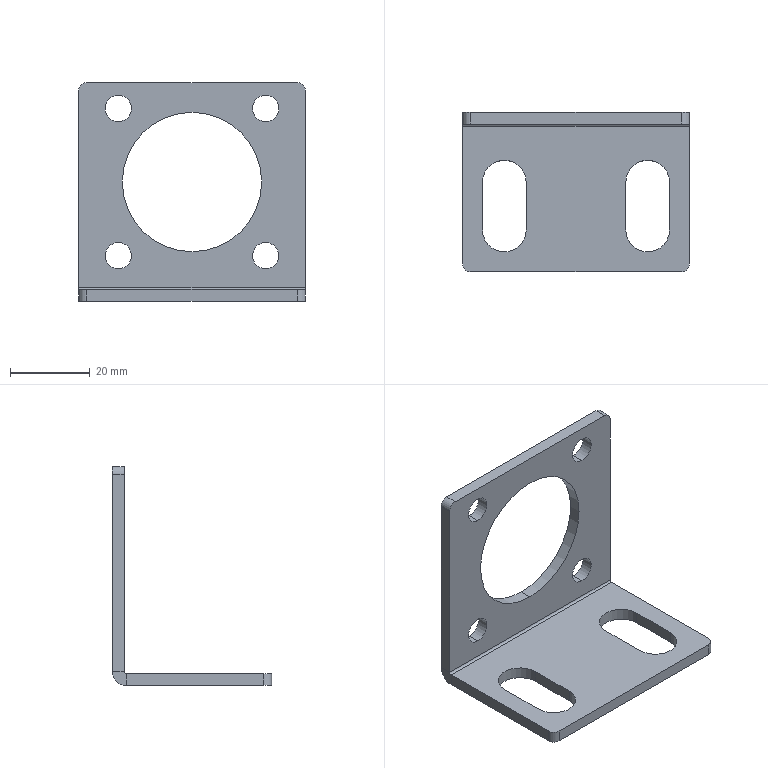Part | SolidWorks | features BaseBody 1 | 1 solid | 36 faces | box 57 x 40 x 55 mm | volume 10916 mm3 | cylinder 20 | plane 16 | commonest cylinder face diameters 6.6 x8 4 x4 11 x4 35 x2 1 x1 7 x1
STEP:
#1=CARTESIAN_POINT('',(0.,17.,9.5));
#2=VERTEX_POINT('',#1);
#3=CARTESIAN_POINT('',(0.,20.,9.5));
#4=VERTEX_POINT('',#3);
#5=CARTESIAN_POINT('',(0.,-20.,9.5));
#6=DIRECTION('',(0.,1.,0.));
#7=VECTOR('',#6,1000.);
#8=LINE('',#5,#7);
#9=EDGE_CURVE('',#2,#4,#8,.T.);
#10=ORIENTED_EDGE('',*,*,#9,.F.);
#11=CARTESIAN_POINT('',(0.,17.,44.5));
#12=VERTEX_POINT('',#11);
#13=CARTESIAN_POINT('',(0.,17.,27.));
#14=DIRECTION('',(0.,1.,0.));
#15=DIRECTION('',(0.,0.,-1.));
#16=AXIS2_PLACEMENT_3D('',#13,#14,#15);
#17=CIRCLE('',#16,17.5);
#18=EDGE_CURVE('',#12,#2,#17,.T.);
#19=ORIENTED_EDGE('',*,*,#18,.F.);
#20=CARTESIAN_POINT('',(0.,20.,44.5));
#21=VERTEX_POINT('',#20);
#22=CARTESIAN_POINT('',(0.,-20.,44.5));
#23=DIRECTION('',(0.,1.,0.));
#24=VECTOR('',#23,1000.);
#25=LINE('',#22,#24);
#26=EDGE_CURVE('',#12,#21,#25,.T.);
#27=ORIENTED_EDGE('',*,*,#26,.T.);
#28=CARTESIAN_POINT('',(0.,20.,27.));
#29=DIRECTION('',(0.,1.,0.));
#30=DIRECTION('',(0.,0.,-1.));
#31=AXIS2_PLACEMENT_3D('',#28,#29,#30);
#32=CIRCLE('',#31,17.5);
#33=EDGE_CURVE('',#21,#4,#32,.T.);
#34=ORIENTED_EDGE('',*,*,#33,.T.);
#35=EDGE_LOOP('',(#10,#19,#27,#34));
#36=FACE_OUTER_BOUND('',#35,.T.);
#37=CARTESIAN_POINT('',(0.,-20.,27.));
#38=DIRECTION('',(0.,1.,0.));
#39=DIRECTION('',(0.,0.,1.));
#40=AXIS2_PLACEMENT_3D('',#37,#38,#39);
#41=CYLINDRICAL_SURFACE('',#40,17.5);
#42=ADVANCED_FACE('',(#36),#41,.F.);
#43=CARTESIAN_POINT('',(-12.5,-9.5,0.));
#44=VERTEX_POINT('',#43);
#45=CARTESIAN_POINT('',(-12.5,-9.5,-3.));
#46=VERTEX_POINT('',#45);
#47=CARTESIAN_POINT('',(-12.5,-9.5,-3.001));
#48=DIRECTION('',(0.,0.,-1.));
#49=VECTOR('',#48,1000.);
#50=LINE('',#47,#49);
#51=EDGE_CURVE('',#44,#46,#50,.T.);
#52=ORIENTED_EDGE('',*,*,#51,.F.);
#53=CARTESIAN_POINT('',(-12.5,2.5,0.));
#54=VERTEX_POINT('',#53);
#55=CARTESIAN_POINT('',(-12.5,-9.5,0.));
#56=DIRECTION('',(0.,1.,0.));
#57=VECTOR('',#56,1000.);
#58=LINE('',#55,#57);
#59=EDGE_CURVE('',#44,#54,#58,.T.);
#60=ORIENTED_EDGE('',*,*,#59,.T.);
#61=CARTESIAN_POINT('',(-12.5,2.5,-3.));
#62=VERTEX_POINT('',#61);
#63=CARTESIAN_POINT('',(-12.5,2.5,-3.001));
#64=DIRECTION('',(0.,0.,-1.));
#65=VECTOR('',#64,1000.);
#66=LINE('',#63,#65);
#67=EDGE_CURVE('',#54,#62,#66,.T.);
#68=ORIENTED_EDGE('',*,*,#67,.T.);
#69=CARTESIAN_POINT('',(-12.5,0.,-3.));
#70=DIRECTION('',(0.,1.,0.));
#71=VECTOR('',#70,1000.);
#72=LINE('',#69,#71);
#73=EDGE_CURVE('',#46,#62,#72,.T.);
#74=ORIENTED_EDGE('',*,*,#73,.F.);
#75=EDGE_LOOP('',(#52,#60,#68,#74));
#76=FACE_OUTER_BOUND('',#75,.T.);
#77=CARTESIAN_POINT('',(-12.5,-9.5,-3.001));
#78=DIRECTION('',(1.,0.,0.));
#79=DIRECTION('',(0.,0.,1.));
#80=AXIS2_PLACEMENT_3D('',#77,#78,#79);
#81=PLANE('',#80);
#82=ADVANCED_FACE('',(#76),#81,.F.);
#83=CARTESIAN_POINT('',(-23.5,2.5,-3.));
#84=VERTEX_POINT('',#83);
#85=CARTESIAN_POINT('',(-23.5,2.5,0.));
#86=VERTEX_POINT('',#85);
#87=CARTESIAN_POINT('',(-23.5,2.5,0.));
#88=DIRECTION('',(0.,0.,1.));
#89=VECTOR('',#88,1000.);
#90=LINE('',#87,#89);
#91=EDGE_CURVE('',#84,#86,#90,.T.);
#92=ORIENTED_EDGE('',*,*,#91,.T.);
#93=CARTESIAN_POINT('',(-23.5,-9.5,0.));
#94=VERTEX_POINT('',#93);
#95=CARTESIAN_POINT('',(-23.5,-9.5,0.));
#96=DIRECTION('',(0.,1.,0.));
#97=VECTOR('',#96,1000.);
#98=LINE('',#95,#97);
#99=EDGE_CURVE('',#94,#86,#98,.T.);
#100=ORIENTED_EDGE('',*,*,#99,.F.);
#101=CARTESIAN_POINT('',(-23.5,-9.5,-3.));
#102=VERTEX_POINT('',#101);
#103=CARTESIAN_POINT('',(-23.5,-9.5,0.));
#104=DIRECTION('',(0.,0.,-1.));
#105=VECTOR('',#104,1000.);
#106=LINE('',#103,#105);
#107=EDGE_CURVE('',#94,#102,#106,.T.);
#108=ORIENTED_EDGE('',*,*,#107,.T.);
#109=CARTESIAN_POINT('',(-23.5,0.,-3.));
#110=DIRECTION('',(0.,-1.,0.));
#111=VECTOR('',#110,1000.);
#112=LINE('',#109,#111);
#113=EDGE_CURVE('',#84,#102,#112,.T.);
#114=ORIENTED_EDGE('',*,*,#113,.F.);
#115=EDGE_LOOP('',(#92,#100,#108,#114));
#116=FACE_OUTER_BOUND('',#115,.T.);
#117=CARTESIAN_POINT('',(-23.5,-9.5,0.));
#118=DIRECTION('',(-1.,0.,0.));
#119=DIRECTION('',(0.,0.,1.));
#120=AXIS2_PLACEMENT_3D('',#117,#118,#119);
#121=PLANE('',#120);
#122=ADVANCED_FACE('',(#116),#121,.F.);
#123=ORIENTED_EDGE('',*,*,#107,.F.);
#124=CARTESIAN_POINT('',(-18.,-9.5,0.));
#125=DIRECTION('',(0.,0.,1.));
#126=DIRECTION('',(1.,0.,0.));
#127=AXIS2_PLACEMENT_3D('',#124,#125,#126);
#128=CIRCLE('',#127,5.5);
#129=EDGE_CURVE('',#94,#44,#128,.T.);
#130=ORIENTED_EDGE('',*,*,#129,.T.);
#131=ORIENTED_EDGE('',*,*,#51,.T.);
#132=CARTESIAN_POINT('',(-18.,-9.5,-3.));
#133=DIRECTION('',(0.,0.,1.));
#134=DIRECTION('',(1.,0.,0.));
#135=AXIS2_PLACEMENT_3D('',#132,#133,#134);
#136=CIRCLE('',#135,5.5);
#137=EDGE_CURVE('',#102,#46,#136,.T.);
#138=ORIENTED_EDGE('',*,*,#137,.F.);
#139=EDGE_LOOP('',(#123,#130,#131,#138));
#140=FACE_OUTER_BOUND('',#139,.T.);
#141=CARTESIAN_POINT('',(-18.,-9.5,0.));
#142=DIRECTION('',(0.,0.,1.));
#143=DIRECTION('',(1.,0.,0.));
#144=AXIS2_PLACEMENT_3D('',#141,#142,#143);
#145=CYLINDRICAL_SURFACE('',#144,5.5);
#146=ADVANCED_FACE('',(#140),#145,.F.);
#147=ORIENTED_EDGE('',*,*,#67,.F.);
#148=CARTESIAN_POINT('',(-18.,2.5,0.));
#149=DIRECTION('',(0.,0.,1.));
#150=DIRECTION('',(1.,0.,0.));
#151=AXIS2_PLACEMENT_3D('',#148,#149,#150);
#152=CIRCLE('',#151,5.5);
#153=EDGE_CURVE('',#54,#86,#152,.T.);
#154=ORIENTED_EDGE('',*,*,#153,.T.);
#155=ORIENTED_EDGE('',*,*,#91,.F.);
#156=CARTESIAN_POINT('',(-18.,2.5,-3.));
#157=DIRECTION('',(0.,0.,1.));
#158=DIRECTION('',(1.,0.,0.));
#159=AXIS2_PLACEMENT_3D('',#156,#157,#158);
#160=CIRCLE('',#159,5.5);
#161=EDGE_CURVE('',#62,#84,#160,.T.);
#162=ORIENTED_EDGE('',*,*,#161,.F.);
#163=EDGE_LOOP('',(#147,#154,#155,#162));
#164=FACE_OUTER_BOUND('',#163,.T.);
#165=CARTESIAN_POINT('',(-18.,2.5,0.));
#166=DIRECTION('',(0.,0.,1.));
#167=DIRECTION('',(1.,0.,0.));
#168=AXIS2_PLACEMENT_3D('',#165,#166,#167);
#169=CYLINDRICAL_SURFACE('',#168,5.5);
#170=ADVANCED_FACE('',(#164),#169,.F.);
#171=CARTESIAN_POINT('',(23.5,-9.5,0.));
#172=VERTEX_POINT('',#171);
#173=CARTESIAN_POINT('',(23.5,-9.5,-3.));
#174=VERTEX_POINT('',#173);
#175=CARTESIAN_POINT('',(23.5,-9.5,-3.001));
#176=DIRECTION('',(0.,0.,-1.));
#177=VECTOR('',#176,1000.);
#178=LINE('',#175,#177);
#179=EDGE_CURVE('',#172,#174,#178,.T.);
#180=ORIENTED_EDGE('',*,*,#179,.F.);
#181=CARTESIAN_POINT('',(23.5,2.5,0.));
#182=VERTEX_POINT('',#181);
#183=CARTESIAN_POINT('',(23.5,-9.5,0.));
#184=DIRECTION('',(0.,1.,0.));
#185=VECTOR('',#184,1000.);
#186=LINE('',#183,#185);
#187=EDGE_CURVE('',#172,#182,#186,.T.);
#188=ORIENTED_EDGE('',*,*,#187,.T.);
#189=CARTESIAN_POINT('',(23.5,2.5,-3.));
#190=VERTEX_POINT('',#189);
#191=CARTESIAN_POINT('',(23.5,2.5,-3.001));
#192=DIRECTION('',(0.,0.,-1.));
#193=VECTOR('',#192,1000.);
#194=LINE('',#191,#193);
#195=EDGE_CURVE('',#182,#190,#194,.T.);
#196=ORIENTED_EDGE('',*,*,#195,.T.);
#197=CARTESIAN_POINT('',(23.5,0.,-3.));
#198=DIRECTION('',(0.,1.,0.));
#199=VECTOR('',#198,1000.);
#200=LINE('',#197,#199);
#201=EDGE_CURVE('',#174,#190,#200,.T.);
#202=ORIENTED_EDGE('',*,*,#201,.F.);
#203=EDGE_LOOP('',(#180,#188,#196,#202));
#204=FACE_OUTER_BOUND('',#203,.T.);
#205=CARTESIAN_POINT('',(23.5,-9.5,-3.001));
#206=DIRECTION('',(1.,0.,0.));
#207=DIRECTION('',(0.,0.,1.));
#208=AXIS2_PLACEMENT_3D('',#205,#206,#207);
#209=PLANE('',#208);
#210=ADVANCED_FACE('',(#204),#209,.F.);
#211=CARTESIAN_POINT('',(12.5,2.5,-3.));
#212=VERTEX_POINT('',#211);
#213=CARTESIAN_POINT('',(12.5,2.5,0.));
#214=VERTEX_POINT('',#213);
#215=CARTESIAN_POINT('',(12.5,2.5,0.));
#216=DIRECTION('',(0.,0.,1.));
#217=VECTOR('',#216,1000.);
#218=LINE('',#215,#217);
#219=EDGE_CURVE('',#212,#214,#218,.T.);
#220=ORIENTED_EDGE('',*,*,#219,.T.);
#221=CARTESIAN_POINT('',(12.5,-9.5,0.));
#222=VERTEX_POINT('',#221);
#223=CARTESIAN_POINT('',(12.5,-9.5,0.));
#224=DIRECTION('',(0.,1.,0.));
#225=VECTOR('',#224,1000.);
#226=LINE('',#223,#225);
#227=EDGE_CURVE('',#222,#214,#226,.T.);
#228=ORIENTED_EDGE('',*,*,#227,.F.);
#229=CARTESIAN_POINT('',(12.5,-9.5,-3.));
#230=VERTEX_POINT('',#229);
#231=CARTESIAN_POINT('',(12.5,-9.5,0.));
#232=DIRECTION('',(0.,0.,-1.));
#233=VECTOR('',#232,1000.);
#234=LINE('',#231,#233);
#235=EDGE_CURVE('',#222,#230,#234,.T.);
#236=ORIENTED_EDGE('',*,*,#235,.T.);
#237=CARTESIAN_POINT('',(12.5,0.,-3.));
#238=DIRECTION('',(0.,-1.,0.));
#239=VECTOR('',#238,1000.);
#240=LINE('',#237,#239);
#241=EDGE_CURVE('',#212,#230,#240,.T.);
#242=ORIENTED_EDGE('',*,*,#241,.F.);
#243=EDGE_LOOP('',(#220,#228,#236,#242));
#244=FACE_OUTER_BOUND('',#243,.T.);
#245=CARTESIAN_POINT('',(12.5,-9.5,0.));
#246=DIRECTION('',(-1.,0.,0.));
#247=DIRECTION('',(0.,0.,1.));
#248=AXIS2_PLACEMENT_3D('',#245,#246,#247);
#249=PLANE('',#248);
#250=ADVANCED_FACE('',(#244),#249,.F.);
#251=ORIENTED_EDGE('',*,*,#235,.F.);
#252=CARTESIAN_POINT('',(18.,-9.5,0.));
#253=DIRECTION('',(0.,0.,1.));
#254=DIRECTION('',(1.,0.,0.));
#255=AXIS2_PLACEMENT_3D('',#252,#253,#254);
#256=CIRCLE('',#255,5.5);
#257=EDGE_CURVE('',#222,#172,#256,.T.);
#258=ORIENTED_EDGE('',*,*,#257,.T.);
#259=ORIENTED_EDGE('',*,*,#179,.T.);
#260=CARTESIAN_POINT('',(18.,-9.5,-3.));
#261=DIRECTION('',(0.,0.,1.));
#262=DIRECTION('',(1.,0.,0.));
#263=AXIS2_PLACEMENT_3D('',#260,#261,#262);
#264=CIRCLE('',#263,5.5);
#265=EDGE_CURVE('',#230,#174,#264,.T.);
#266=ORIENTED_EDGE('',*,*,#265,.F.);
#267=EDGE_LOOP('',(#251,#258,#259,#266));
#268=FACE_OUTER_BOUND('',#267,.T.);
#269=CARTESIAN_POINT('',(18.,-9.5,0.));
#270=DIRECTION('',(0.,0.,1.));
#271=DIRECTION('',(1.,0.,0.));
#272=AXIS2_PLACEMENT_3D('',#269,#270,#271);
#273=CYLINDRICAL_SURFACE('',#272,5.5);
#274=ADVANCED_FACE('',(#268),#273,.F.);
#275=ORIENTED_EDGE('',*,*,#195,.F.);
#276=CARTESIAN_POINT('',(18.,2.5,0.));
#277=DIRECTION('',(0.,0.,1.));
#278=DIRECTION('',(1.,0.,0.));
#279=AXIS2_PLACEMENT_3D('',#276,#277,#278);
#280=CIRCLE('',#279,5.5);
#281=EDGE_CURVE('',#182,#214,#280,.T.);
#282=ORIENTED_EDGE('',*,*,#281,.T.);
#283=ORIENTED_EDGE('',*,*,#219,.F.);
#284=CARTESIAN_POINT('',(18.,2.5,-3.));
#285=DIRECTION('',(0.,0.,1.));
#286=DIRECTION('',(1.,0.,0.));
#287=AXIS2_PLACEMENT_3D('',#284,#285,#286);
#288=CIRCLE('',#287,5.5);
#289=EDGE_CURVE('',#190,#212,#288,.T.);
#290=ORIENTED_EDGE('',*,*,#289,.F.);
#291=EDGE_LOOP('',(#275,#282,#283,#290));
#292=FACE_OUTER_BOUND('',#291,.T.);
#293=CARTESIAN_POINT('',(18.,2.5,0.));
#294=DIRECTION('',(0.,0.,1.));
#295=DIRECTION('',(1.,0.,0.));
#296=AXIS2_PLACEMENT_3D('',#293,#294,#295);
#297=CYLINDRICAL_SURFACE('',#296,5.5);
#298=ADVANCED_FACE('',(#292),#297,.F.);
#299=CARTESIAN_POINT('',(18.5,20.,11.8));
#300=VERTEX_POINT('',#299);
#301=CARTESIAN_POINT('',(18.5,17.,11.8));
#302=VERTEX_POINT('',#301);
#303=CARTESIAN_POINT('',(18.5,17.,11.8));
#304=DIRECTION('',(0.,-1.,0.));
#305=VECTOR('',#304,1000.);
#306=LINE('',#303,#305);
#307=EDGE_CURVE('',#300,#302,#306,.T.);
#308=ORIENTED_EDGE('',*,*,#307,.F.);
#309=CARTESIAN_POINT('',(18.5,20.,5.2));
#310=VERTEX_POINT('',#309);
#311=CARTESIAN_POINT('',(18.5,20.,8.5));
#312=DIRECTION('',(0.,-1.,0.));
#313=DIRECTION('',(0.,0.,-1.));
#314=AXIS2_PLACEMENT_3D('',#311,#312,#313);
#315=CIRCLE('',#314,3.3);
#316=EDGE_CURVE('',#310,#300,#315,.T.);
#317=ORIENTED_EDGE('',*,*,#316,.F.);
#318=CARTESIAN_POINT('',(18.5,17.,5.2));
#319=VERTEX_POINT('',#318);
#320=CARTESIAN_POINT('',(18.5,17.,5.2));
#321=DIRECTION('',(0.,-1.,0.));
#322=VECTOR('',#321,1000.);
#323=LINE('',#320,#322);
#324=EDGE_CURVE('',#310,#319,#323,.T.);
#325=ORIENTED_EDGE('',*,*,#324,.T.);
#326=CARTESIAN_POINT('',(18.5,17.,8.5));
#327=DIRECTION('',(0.,-1.,0.));
#328=DIRECTION('',(0.,0.,-1.));
#329=AXIS2_PLACEMENT_3D('',#326,#327,#328);
#330=CIRCLE('',#329,3.3);
#331=EDGE_CURVE('',#319,#302,#330,.T.);
#332=ORIENTED_EDGE('',*,*,#331,.T.);
#333=EDGE_LOOP('',(#308,#317,#325,#332));
#334=FACE_OUTER_BOUND('',#333,.T.);
#335=CARTESIAN_POINT('',(18.5,17.,8.5));
#336=DIRECTION('',(0.,-1.,0.));
#337=DIRECTION('',(0.,0.,-1.));
#338=AXIS2_PLACEMENT_3D('',#335,#336,#337);
#339=CYLINDRICAL_SURFACE('',#338,3.3);
#340=ADVANCED_FACE('',(#334),#339,.F.);
#341=CARTESIAN_POINT('',(-18.5,20.,11.8));
#342=VERTEX_POINT('',#341);
#343=CARTESIAN_POINT('',(-18.5,17.,11.8));
#344=VERTEX_POINT('',#343);
#345=CARTESIAN_POINT('',(-18.5,17.,11.8));
#346=DIRECTION('',(0.,-1.,0.));
#347=VECTOR('',#346,1000.);
#348=LINE('',#345,#347);
#349=EDGE_CURVE('',#342,#344,#348,.T.);
#350=ORIENTED_EDGE('',*,*,#349,.F.);
#351=CARTESIAN_POINT('',(-18.5,20.,5.2));
#352=VERTEX_POINT('',#351);
#353=CARTESIAN_POINT('',(-18.5,20.,8.5));
#354=DIRECTION('',(0.,-1.,0.));
#355=DIRECTION('',(0.,0.,-1.));
#356=AXIS2_PLACEMENT_3D('',#353,#354,#355);
#357=CIRCLE('',#356,3.3);
#358=EDGE_CURVE('',#352,#342,#357,.T.);
#359=ORIENTED_EDGE('',*,*,#358,.F.);
#360=CARTESIAN_POINT('',(-18.5,17.,5.2));
#361=VERTEX_POINT('',#360);
#362=CARTESIAN_POINT('',(-18.5,17.,5.2));
#363=DIRECTION('',(0.,-1.,0.));
#364=VECTOR('',#363,1000.);
#365=LINE('',#362,#364);
#366=EDGE_CURVE('',#352,#361,#365,.T.);
#367=ORIENTED_EDGE('',*,*,#366,.T.);
#368=CARTESIAN_POINT('',(-18.5,17.,8.5));
#369=DIRECTION('',(0.,-1.,0.));
#370=DIRECTION('',(0.,0.,-1.));
#371=AXIS2_PLACEMENT_3D('',#368,#369,#370);
#372=CIRCLE('',#371,3.3);
#373=EDGE_CURVE('',#361,#344,#372,.T.);
#374=ORIENTED_EDGE('',*,*,#373,.T.);
#375=EDGE_LOOP('',(#350,#359,#367,#374));
#376=FACE_OUTER_BOUND('',#375,.T.);
#377=CARTESIAN_POINT('',(-18.5,17.,8.5));
#378=DIRECTION('',(0.,-1.,0.));
#379=DIRECTION('',(0.,0.,-1.));
#380=AXIS2_PLACEMENT_3D('',#377,#378,#379);
#381=CYLINDRICAL_SURFACE('',#380,3.3);
#382=ADVANCED_FACE('',(#376),#381,.F.);
#383=CARTESIAN_POINT('',(-18.5,20.,48.8));
#384=VERTEX_POINT('',#383);
#385=CARTESIAN_POINT('',(-18.5,17.,48.8));
#386=VERTEX_POINT('',#385);
#387=CARTESIAN_POINT('',(-18.5,17.,48.8));
#388=DIRECTION('',(0.,-1.,0.));
#389=VECTOR('',#388,1000.);
#390=LINE('',#387,#389);
#391=EDGE_CURVE('',#384,#386,#390,.T.);
#392=ORIENTED_EDGE('',*,*,#391,.F.);
#393=CARTESIAN_POINT('',(-18.5,20.,42.2));
#394=VERTEX_POINT('',#393);
#395=CARTESIAN_POINT('',(-18.5,20.,45.5));
#396=DIRECTION('',(0.,-1.,0.));
#397=DIRECTION('',(0.,0.,-1.));
#398=AXIS2_PLACEMENT_3D('',#395,#396,#397);
#399=CIRCLE('',#398,3.3);
#400=EDGE_CURVE('',#394,#384,#399,.T.);
#401=ORIENTED_EDGE('',*,*,#400,.F.);
#402=CARTESIAN_POINT('',(-18.5,17.,42.2));
#403=VERTEX_POINT('',#402);
#404=CARTESIAN_POINT('',(-18.5,17.,42.2));
#405=DIRECTION('',(0.,-1.,0.));
#406=VECTOR('',#405,1000.);
#407=LINE('',#404,#406);
#408=EDGE_CURVE('',#394,#403,#407,.T.);
#409=ORIENTED_EDGE('',*,*,#408,.T.);
#410=CARTESIAN_POINT('',(-18.5,17.,45.5));
#411=DIRECTION('',(0.,-1.,0.));
#412=DIRECTION('',(0.,0.,-1.));
#413=AXIS2_PLACEMENT_3D('',#410,#411,#412);
#414=CIRCLE('',#413,3.3);
#415=EDGE_CURVE('',#403,#386,#414,.T.);
#416=ORIENTED_EDGE('',*,*,#415,.T.);
#417=EDGE_LOOP('',(#392,#401,#409,#416));
#418=FACE_OUTER_BOUND('',#417,.T.);
#419=CARTESIAN_POINT('',(-18.5,17.,45.5));
#420=DIRECTION('',(0.,-1.,0.));
#421=DIRECTION('',(0.,0.,-1.));
#422=AXIS2_PLACEMENT_3D('',#419,#420,#421);
#423=CYLINDRICAL_SURFACE('',#422,3.3);
#424=ADVANCED_FACE('',(#418),#423,.F.);
#425=CARTESIAN_POINT('',(18.5,20.,48.8));
#426=VERTEX_POINT('',#425);
#427=CARTESIAN_POINT('',(18.5,17.,48.8));
#428=VERTEX_POINT('',#427);
#429=CARTESIAN_POINT('',(18.5,17.,48.8));
#430=DIRECTION('',(0.,-1.,0.));
#431=VECTOR('',#430,1000.);
#432=LINE('',#429,#431);
#433=EDGE_CURVE('',#426,#428,#432,.T.);
#434=ORIENTED_EDGE('',*,*,#433,.F.);
#435=CARTESIAN_POINT('',(18.5,20.,42.2));
#436=VERTEX_POINT('',#435);
#437=CARTESIAN_POINT('',(18.5,20.,45.5));
#438=DIRECTION('',(0.,-1.,0.));
#439=DIRECTION('',(0.,0.,-1.));
#440=AXIS2_PLACEMENT_3D('',#437,#438,#439);
#441=CIRCLE('',#440,3.3);
#442=EDGE_CURVE('',#436,#426,#441,.T.);
#443=ORIENTED_EDGE('',*,*,#442,.F.);
#444=CARTESIAN_POINT('',(18.5,17.,42.2));
#445=VERTEX_POINT('',#444);
#446=CARTESIAN_POINT('',(18.5,17.,42.2));
#447=DIRECTION('',(0.,-1.,0.));
#448=VECTOR('',#447,1000.);
#449=LINE('',#446,#448);
#450=EDGE_CURVE('',#436,#445,#449,.T.);
#451=ORIENTED_EDGE('',*,*,#450,.T.);
#452=CARTESIAN_POINT('',(18.5,17.,45.5));
#453=DIRECTION('',(0.,-1.,0.));
#454=DIRECTION('',(0.,0.,-1.));
#455=AXIS2_PLACEMENT_3D('',#452,#453,#454);
#456=CIRCLE('',#455,3.3);
#457=EDGE_CURVE('',#445,#428,#456,.T.);
#458=ORIENTED_EDGE('',*,*,#457,.T.);
#459=EDGE_LOOP('',(#434,#443,#451,#458));
#460=FACE_OUTER_BOUND('',#459,.T.);
#461=CARTESIAN_POINT('',(18.5,17.,45.5));
#462=DIRECTION('',(0.,-1.,0.));
#463=DIRECTION('',(0.,0.,-1.));
#464=AXIS2_PLACEMENT_3D('',#461,#462,#463);
#465=CYLINDRICAL_SURFACE('',#464,3.3);
#466=ADVANCED_FACE('',(#460),#465,.F.);
#467=CARTESIAN_POINT('',(-28.5,20.,50.));
#468=VERTEX_POINT('',#467);
#469=CARTESIAN_POINT('',(-26.5,20.,52.));
#470=VERTEX_POINT('',#469);
#471=CARTESIAN_POINT('',(-26.5,20.,50.));
#472=DIRECTION('',(0.,1.,0.));
#473=DIRECTION('',(0.,0.,-1.));
#474=AXIS2_PLACEMENT_3D('',#471,#472,#473);
#475=CIRCLE('',#474,2.);
#476=EDGE_CURVE('',#468,#470,#475,.T.);
#477=ORIENTED_EDGE('',*,*,#476,.F.);
#478=CARTESIAN_POINT('',(-28.5,17.,50.));
#479=VERTEX_POINT('',#478);
#480=CARTESIAN_POINT('',(-28.5,20.,50.));
#481=DIRECTION('',(0.,1.,0.));
#482=VECTOR('',#481,1000.);
#483=LINE('',#480,#482);
#484=EDGE_CURVE('',#479,#468,#483,.T.);
#485=ORIENTED_EDGE('',*,*,#484,.F.);
#486=CARTESIAN_POINT('',(-26.5,17.,52.));
#487=VERTEX_POINT('',#486);
#488=CARTESIAN_POINT('',(-26.5,17.,50.));
#489=DIRECTION('',(0.,-1.,0.));
#490=DIRECTION('',(0.,0.,-1.));
#491=AXIS2_PLACEMENT_3D('',#488,#489,#490);
#492=CIRCLE('',#491,2.);
#493=EDGE_CURVE('',#487,#479,#492,.T.);
#494=ORIENTED_EDGE('',*,*,#493,.F.);
#495=CARTESIAN_POINT('',(-26.5,20.,52.));
#496=DIRECTION('',(0.,-1.,0.));
#497=VECTOR('',#496,1000.);
#498=LINE('',#495,#497);
#499=EDGE_CURVE('',#470,#487,#498,.T.);
#500=ORIENTED_EDGE('',*,*,#499,.F.);
#501=EDGE_LOOP('',(#477,#485,#494,#500));
#502=FACE_OUTER_BOUND('',#501,.T.);
#503=CARTESIAN_POINT('',(-26.5,20.,50.));
#504=DIRECTION('',(0.,-1.,0.));
#505=DIRECTION('',(0.,0.,-1.));
#506=AXIS2_PLACEMENT_3D('',#503,#504,#505);
#507=CYLINDRICAL_SURFACE('',#506,2.);
#508=ADVANCED_FACE('',(#502),#507,.T.);
#509=CARTESIAN_POINT('',(26.5,20.,52.));
#510=VERTEX_POINT('',#509);
#511=CARTESIAN_POINT('',(28.5,20.,50.));
#512=VERTEX_POINT('',#511);
#513=CARTESIAN_POINT('',(26.5,20.,50.));
#514=DIRECTION('',(0.,1.,0.));
#515=DIRECTION('',(0.,0.,-1.));
#516=AXIS2_PLACEMENT_3D('',#513,#514,#515);
#517=CIRCLE('',#516,2.);
#518=EDGE_CURVE('',#510,#512,#517,.T.);
#519=ORIENTED_EDGE('',*,*,#518,.F.);
#520=CARTESIAN_POINT('',(26.5,17.,52.));
#521=VERTEX_POINT('',#520);
#522=CARTESIAN_POINT('',(26.5,20.,52.));
#523=DIRECTION('',(0.,1.,0.));
#524=VECTOR('',#523,1000.);
#525=LINE('',#522,#524);
#526=EDGE_CURVE('',#521,#510,#525,.T.);
#527=ORIENTED_EDGE('',*,*,#526,.F.);
#528=CARTESIAN_POINT('',(28.5,17.,50.));
#529=VERTEX_POINT('',#528);
#530=CARTESIAN_POINT('',(26.5,17.,50.));
#531=DIRECTION('',(0.,-1.,0.));
#532=DIRECTION('',(0.,0.,-1.));
#533=AXIS2_PLACEMENT_3D('',#530,#531,#532);
#534=CIRCLE('',#533,2.);
#535=EDGE_CURVE('',#529,#521,#534,.T.);
#536=ORIENTED_EDGE('',*,*,#535,.F.);
#537=CARTESIAN_POINT('',(28.5,20.,50.));
#538=DIRECTION('',(0.,-1.,0.));
#539=VECTOR('',#538,1000.);
#540=LINE('',#537,#539);
#541=EDGE_CURVE('',#512,#529,#540,.T.);
#542=ORIENTED_EDGE('',*,*,#541,.F.);
#543=EDGE_LOOP('',(#519,#527,#536,#542));
#544=FACE_OUTER_BOUND('',#543,.T.);
#545=CARTESIAN_POINT('',(26.5,20.,50.));
#546=DIRECTION('',(0.,-1.,0.));
#547=DIRECTION('',(0.,0.,-1.));
#548=AXIS2_PLACEMENT_3D('',#545,#546,#547);
#549=CYLINDRICAL_SURFACE('',#548,2.);
#550=ADVANCED_FACE('',(#544),#549,.T.);
#551=CARTESIAN_POINT('',(28.5,-18.,-3.));
#552=VERTEX_POINT('',#551);
#553=CARTESIAN_POINT('',(26.5,-20.,-3.));
#554=VERTEX_POINT('',#553);
#555=CARTESIAN_POINT('',(26.5,-18.,-3.));
#556=DIRECTION('',(0.,0.,-1.));
#557=DIRECTION('',(1.,0.,0.));
#558=AXIS2_PLACEMENT_3D('',#555,#556,#557);
#559=CIRCLE('',#558,2.);
#560=EDGE_CURVE('',#552,#554,#559,.T.);
#561=ORIENTED_EDGE('',*,*,#560,.F.);
#562=CARTESIAN_POINT('',(28.5,-18.,0.));
#563=VERTEX_POINT('',#562);
#564=CARTESIAN_POINT('',(28.5,-18.,-3.));
#565=DIRECTION('',(0.,0.,-1.));
#566=VECTOR('',#565,1000.);
#567=LINE('',#564,#566);
#568=EDGE_CURVE('',#563,#552,#567,.T.);
#569=ORIENTED_EDGE('',*,*,#568,.F.);
#570=CARTESIAN_POINT('',(26.5,-20.,0.));
#571=VERTEX_POINT('',#570);
#572=CARTESIAN_POINT('',(26.5,-18.,0.));
#573=DIRECTION('',(0.,0.,1.));
#574=DIRECTION('',(1.,0.,0.));
#575=AXIS2_PLACEMENT_3D('',#572,#573,#574);
#576=CIRCLE('',#575,2.);
#577=EDGE_CURVE('',#571,#563,#576,.T.);
#578=ORIENTED_EDGE('',*,*,#577,.F.);
#579=CARTESIAN_POINT('',(26.5,-20.,-3.));
#580=DIRECTION('',(0.,0.,1.));
#581=VECTOR('',#580,1000.);
#582=LINE('',#579,#581);
#583=EDGE_CURVE('',#554,#571,#582,.T.);
#584=ORIENTED_EDGE('',*,*,#583,.F.);
#585=EDGE_LOOP('',(#561,#569,#578,#584));
#586=FACE_OUTER_BOUND('',#585,.T.);
#587=CARTESIAN_POINT('',(26.5,-18.,-3.));
#588=DIRECTION('',(0.,0.,1.));
#589=DIRECTION('',(1.,0.,0.));
#590=AXIS2_PLACEMENT_3D('',#587,#588,#589);
#591=CYLINDRICAL_SURFACE('',#590,2.);
#592=ADVANCED_FACE('',(#586),#591,.T.);
#593=CARTESIAN_POINT('',(-26.5,-20.,-3.));
#594=VERTEX_POINT('',#593);
#595=CARTESIAN_POINT('',(-28.5,-18.,-3.));
#596=VERTEX_POINT('',#595);
#597=CARTESIAN_POINT('',(-26.5,-18.,-3.));
#598=DIRECTION('',(0.,0.,-1.));
#599=DIRECTION('',(1.,0.,0.));
#600=AXIS2_PLACEMENT_3D('',#597,#598,#599);
#601=CIRCLE('',#600,2.);
#602=EDGE_CURVE('',#594,#596,#601,.T.);
#603=ORIENTED_EDGE('',*,*,#602,.F.);
#604=CARTESIAN_POINT('',(-26.5,-20.,0.));
#605=VERTEX_POINT('',#604);
#606=CARTESIAN_POINT('',(-26.5,-20.,-3.));
#607=DIRECTION('',(0.,0.,-1.));
#608=VECTOR('',#607,1000.);
#609=LINE('',#606,#608);
#610=EDGE_CURVE('',#605,#594,#609,.T.);
#611=ORIENTED_EDGE('',*,*,#610,.F.);
#612=CARTESIAN_POINT('',(-28.5,-18.,0.));
#613=VERTEX_POINT('',#612);
#614=CARTESIAN_POINT('',(-26.5,-18.,0.));
#615=DIRECTION('',(0.,0.,1.));
#616=DIRECTION('',(1.,0.,0.));
#617=AXIS2_PLACEMENT_3D('',#614,#615,#616);
#618=CIRCLE('',#617,2.);
#619=EDGE_CURVE('',#613,#605,#618,.T.);
#620=ORIENTED_EDGE('',*,*,#619,.F.);
#621=CARTESIAN_POINT('',(-28.5,-18.,-3.));
#622=DIRECTION('',(0.,0.,1.));
#623=VECTOR('',#622,1000.);
#624=LINE('',#621,#623);
#625=EDGE_CURVE('',#596,#613,#624,.T.);
#626=ORIENTED_EDGE('',*,*,#625,.F.);
#627=EDGE_LOOP('',(#603,#611,#620,#626));
#628=FACE_OUTER_BOUND('',#627,.T.);
#629=CARTESIAN_POINT('',(-26.5,-18.,-3.));
#630=DIRECTION('',(0.,0.,1.));
#631=DIRECTION('',(1.,0.,0.));
#632=AXIS2_PLACEMENT_3D('',#629,#630,#631);
#633=CYLINDRICAL_SURFACE('',#632,2.);
#634=ADVANCED_FACE('',(#628),#633,.T.);
#635=CARTESIAN_POINT('',(28.5,17.,52.));
#636=DIRECTION('',(1.,0.,0.));
#637=VECTOR('',#636,1000.);
#638=LINE('',#635,#637);
#639=EDGE_CURVE('',#487,#521,#638,.T.);
#640=ORIENTED_EDGE('',*,*,#639,.T.);
#641=ORIENTED_EDGE('',*,*,#526,.T.);
#642=CARTESIAN_POINT('',(0.,20.,52.));
#643=DIRECTION('',(1.,0.,0.));
#644=VECTOR('',#643,1000.);
#645=LINE('',#642,#644);
#646=EDGE_CURVE('',#470,#510,#645,.T.);
#647=ORIENTED_EDGE('',*,*,#646,.F.);
#648=ORIENTED_EDGE('',*,*,#499,.T.);
#649=EDGE_LOOP('',(#640,#641,#647,#648));
#650=FACE_OUTER_BOUND('',#649,.T.);
#651=CARTESIAN_POINT('',(28.5,20.,52.));
#652=DIRECTION('',(0.,0.,-1.));
#653=DIRECTION('',(0.,-1.,0.));
#654=AXIS2_PLACEMENT_3D('',#651,#652,#653);
#655=PLANE('',#654);
#656=ADVANCED_FACE('',(#650),#655,.F.);
#657=ORIENTED_EDGE('',*,*,#457,.F.);
#658=CARTESIAN_POINT('',(18.5,17.,45.5));
#659=DIRECTION('',(0.,-1.,0.));
#660=DIRECTION('',(0.,0.,-1.));
#661=AXIS2_PLACEMENT_3D('',#658,#659,#660);
#662=CIRCLE('',#661,3.3);
#663=EDGE_CURVE('',#428,#445,#662,.T.);
#664=ORIENTED_EDGE('',*,*,#663,.F.);
#665=EDGE_LOOP('',(#657,#664));
#666=FACE_BOUND('',#665,.T.);
#667=ORIENTED_EDGE('',*,*,#415,.F.);
#668=CARTESIAN_POINT('',(-18.5,17.,45.5));
#669=DIRECTION('',(0.,-1.,0.));
#670=DIRECTION('',(0.,0.,-1.));
#671=AXIS2_PLACEMENT_3D('',#668,#669,#670);
#672=CIRCLE('',#671,3.3);
#673=EDGE_CURVE('',#386,#403,#672,.T.);
#674=ORIENTED_EDGE('',*,*,#673,.F.);
#675=EDGE_LOOP('',(#667,#674));
#676=FACE_BOUND('',#675,.T.);
#677=ORIENTED_EDGE('',*,*,#373,.F.);
#678=CARTESIAN_POINT('',(-18.5,17.,8.5));
#679=DIRECTION('',(0.,-1.,0.));
#680=DIRECTION('',(0.,0.,-1.));
#681=AXIS2_PLACEMENT_3D('',#678,#679,#680);
#682=CIRCLE('',#681,3.3);
#683=EDGE_CURVE('',#344,#361,#682,.T.);
#684=ORIENTED_EDGE('',*,*,#683,.F.);
#685=EDGE_LOOP('',(#677,#684));
#686=FACE_BOUND('',#685,.T.);
#687=ORIENTED_EDGE('',*,*,#331,.F.);
#688=CARTESIAN_POINT('',(18.5,17.,8.5));
#689=DIRECTION('',(0.,-1.,0.));
#690=DIRECTION('',(0.,0.,-1.));
#691=AXIS2_PLACEMENT_3D('',#688,#689,#690);
#692=CIRCLE('',#691,3.3);
#693=EDGE_CURVE('',#302,#319,#692,.T.);
#694=ORIENTED_EDGE('',*,*,#693,.F.);
#695=EDGE_LOOP('',(#687,#694));
#696=FACE_BOUND('',#695,.T.);
#697=ORIENTED_EDGE('',*,*,#18,.T.);
#698=CARTESIAN_POINT('',(0.,17.,27.));
#699=DIRECTION('',(0.,1.,0.));
#700=DIRECTION('',(0.,0.,-1.));
#701=AXIS2_PLACEMENT_3D('',#698,#699,#700);
#702=CIRCLE('',#701,17.5);
#703=EDGE_CURVE('',#2,#12,#702,.T.);
#704=ORIENTED_EDGE('',*,*,#703,.T.);
#705=EDGE_LOOP('',(#697,#704));
#706=FACE_BOUND('',#705,.T.);
#707=CARTESIAN_POINT('',(28.5,17.,0.5));
#708=VERTEX_POINT('',#707);
#709=CARTESIAN_POINT('',(28.5,17.,0.));
#710=DIRECTION('',(0.,0.,-1.));
#711=VECTOR('',#710,1000.);
#712=LINE('',#709,#711);
#713=EDGE_CURVE('',#529,#708,#712,.T.);
#714=ORIENTED_EDGE('',*,*,#713,.F.);
#715=ORIENTED_EDGE('',*,*,#535,.T.);
#716=ORIENTED_EDGE('',*,*,#639,.F.);
#717=ORIENTED_EDGE('',*,*,#493,.T.);
#718=CARTESIAN_POINT('',(-28.5,17.,0.5));
#719=VERTEX_POINT('',#718);
#720=CARTESIAN_POINT('',(-28.5,17.,52.));
#721=DIRECTION('',(0.,0.,1.));
#722=VECTOR('',#721,1000.);
#723=LINE('',#720,#722);
#724=EDGE_CURVE('',#719,#479,#723,.T.);
#725=ORIENTED_EDGE('',*,*,#724,.F.);
#726=CARTESIAN_POINT('',(28.5,17.,0.5));
#727=DIRECTION('',(-1.,0.,0.));
#728=VECTOR('',#727,1000.);
#729=LINE('',#726,#728);
#730=EDGE_CURVE('',#708,#719,#729,.T.);
#731=ORIENTED_EDGE('',*,*,#730,.F.);
#732=EDGE_LOOP('',(#714,#715,#716,#717,#725,#731));
#733=FACE_OUTER_BOUND('',#732,.T.);
#734=CARTESIAN_POINT('',(0.,17.,0.));
#735=DIRECTION('',(0.,-1.,0.));
#736=DIRECTION('',(-1.,0.,0.));
#737=AXIS2_PLACEMENT_3D('',#734,#735,#736);
#738=PLANE('',#737);
#739=ADVANCED_FACE('',(#666,#676,#686,#696,#706,#733),#738,.T.);
#740=ORIENTED_EDGE('',*,*,#442,.T.);
#741=CARTESIAN_POINT('',(18.5,20.,45.5));
#742=DIRECTION('',(0.,-1.,0.));
#743=DIRECTION('',(0.,0.,-1.));
#744=AXIS2_PLACEMENT_3D('',#741,#742,#743);
#745=CIRCLE('',#744,3.3);
#746=EDGE_CURVE('',#426,#436,#745,.T.);
#747=ORIENTED_EDGE('',*,*,#746,.T.);
#748=EDGE_LOOP('',(#740,#747));
#749=FACE_BOUND('',#748,.T.);
#750=ORIENTED_EDGE('',*,*,#400,.T.);
#751=CARTESIAN_POINT('',(-18.5,20.,45.5));
#752=DIRECTION('',(0.,-1.,0.));
#753=DIRECTION('',(0.,0.,-1.));
#754=AXIS2_PLACEMENT_3D('',#751,#752,#753);
#755=CIRCLE('',#754,3.3);
#756=EDGE_CURVE('',#384,#394,#755,.T.);
#757=ORIENTED_EDGE('',*,*,#756,.T.);
#758=EDGE_LOOP('',(#750,#757));
#759=FACE_BOUND('',#758,.T.);
#760=ORIENTED_EDGE('',*,*,#358,.T.);
#761=CARTESIAN_POINT('',(-18.5,20.,8.5));
#762=DIRECTION('',(0.,-1.,0.));
#763=DIRECTION('',(0.,0.,-1.));
#764=AXIS2_PLACEMENT_3D('',#761,#762,#763);
#765=CIRCLE('',#764,3.3);
#766=EDGE_CURVE('',#342,#352,#765,.T.);
#767=ORIENTED_EDGE('',*,*,#766,.T.);
#768=EDGE_LOOP('',(#760,#767));
#769=FACE_BOUND('',#768,.T.);
#770=ORIENTED_EDGE('',*,*,#316,.T.);
#771=CARTESIAN_POINT('',(18.5,20.,8.5));
#772=DIRECTION('',(0.,-1.,0.));
#773=DIRECTION('',(0.,0.,-1.));
#774=AXIS2_PLACEMENT_3D('',#771,#772,#773);
#775=CIRCLE('',#774,3.3);
#776=EDGE_CURVE('',#300,#310,#775,.T.);
#777=ORIENTED_EDGE('',*,*,#776,.T.);
#778=EDGE_LOOP('',(#770,#777));
#779=FACE_BOUND('',#778,.T.);
#780=ORIENTED_EDGE('',*,*,#33,.F.);
#781=CARTESIAN_POINT('',(0.,20.,27.));
#782=DIRECTION('',(0.,1.,0.));
#783=DIRECTION('',(0.,0.,-1.));
#784=AXIS2_PLACEMENT_3D('',#781,#782,#783);
#785=CIRCLE('',#784,17.5);
#786=EDGE_CURVE('',#4,#21,#785,.T.);
#787=ORIENTED_EDGE('',*,*,#786,.F.);
#788=EDGE_LOOP('',(#780,#787));
#789=FACE_BOUND('',#788,.T.);
#790=ORIENTED_EDGE('',*,*,#646,.T.);
#791=ORIENTED_EDGE('',*,*,#518,.T.);
#792=CARTESIAN_POINT('',(28.5,20.,0.5));
#793=VERTEX_POINT('',#792);
#794=CARTESIAN_POINT('',(28.5,20.,0.));
#795=DIRECTION('',(0.,0.,-1.));
#796=VECTOR('',#795,1000.);
#797=LINE('',#794,#796);
#798=EDGE_CURVE('',#512,#793,#797,.T.);
#799=ORIENTED_EDGE('',*,*,#798,.T.);
#800=CARTESIAN_POINT('',(-28.5,20.,0.5));
#801=VERTEX_POINT('',#800);
#802=CARTESIAN_POINT('',(28.5,20.,0.5));
#803=DIRECTION('',(1.,0.,0.));
#804=VECTOR('',#803,1000.);
#805=LINE('',#802,#804);
#806=EDGE_CURVE('',#801,#793,#805,.T.);
#807=ORIENTED_EDGE('',*,*,#806,.F.);
#808=CARTESIAN_POINT('',(-28.5,20.,0.));
#809=DIRECTION('',(0.,0.,1.));
#810=VECTOR('',#809,1000.);
#811=LINE('',#808,#810);
#812=EDGE_CURVE('',#801,#468,#811,.T.);
#813=ORIENTED_EDGE('',*,*,#812,.T.);
#814=ORIENTED_EDGE('',*,*,#476,.T.);
#815=EDGE_LOOP('',(#790,#791,#799,#807,#813,#814));
#816=FACE_OUTER_BOUND('',#815,.T.);
#817=CARTESIAN_POINT('',(0.,20.,0.));
#818=DIRECTION('',(0.,-1.,0.));
#819=DIRECTION('',(-1.,0.,0.));
#820=AXIS2_PLACEMENT_3D('',#817,#818,#819);
#821=PLANE('',#820);
#822=ADVANCED_FACE('',(#749,#759,#769,#779,#789,#816),#821,.F.);
#823=ORIENTED_EDGE('',*,*,#724,.T.);
#824=ORIENTED_EDGE('',*,*,#484,.T.);
#825=ORIENTED_EDGE('',*,*,#812,.F.);
#826=CARTESIAN_POINT('',(-28.5,17.,0.5));
#827=DIRECTION('',(0.,1.,0.));
#828=VECTOR('',#827,1000.);
#829=LINE('',#826,#828);
#830=EDGE_CURVE('',#719,#801,#829,.T.);
#831=ORIENTED_EDGE('',*,*,#830,.F.);
#832=EDGE_LOOP('',(#823,#824,#825,#831));
#833=FACE_OUTER_BOUND('',#832,.T.);
#834=CARTESIAN_POINT('',(-28.5,20.,52.));
#835=DIRECTION('',(1.,0.,0.));
#836=DIRECTION('',(0.,0.,1.));
#837=AXIS2_PLACEMENT_3D('',#834,#835,#836);
#838=PLANE('',#837);
#839=ADVANCED_FACE('',(#833),#838,.F.);
#840=ORIENTED_EDGE('',*,*,#798,.F.);
#841=ORIENTED_EDGE('',*,*,#541,.T.);
#842=ORIENTED_EDGE('',*,*,#713,.T.);
#843=CARTESIAN_POINT('',(28.5,20.,0.5));
#844=DIRECTION('',(0.,1.,0.));
#845=VECTOR('',#844,1000.);
#846=LINE('',#843,#845);
#847=EDGE_CURVE('',#708,#793,#846,.T.);
#848=ORIENTED_EDGE('',*,*,#847,.T.);
#849=EDGE_LOOP('',(#840,#841,#842,#848));
#850=FACE_OUTER_BOUND('',#849,.T.);
#851=CARTESIAN_POINT('',(28.5,20.,0.));
#852=DIRECTION('',(-1.,0.,0.));
#853=DIRECTION('',(0.,0.,1.));
#854=AXIS2_PLACEMENT_3D('',#851,#852,#853);
#855=PLANE('',#854);
#856=ADVANCED_FACE('',(#850),#855,.F.);
#857=CARTESIAN_POINT('',(-28.5,16.5,0.));
#858=VERTEX_POINT('',#857);
#859=CARTESIAN_POINT('',(28.5,16.5,0.));
#860=VERTEX_POINT('',#859);
#861=CARTESIAN_POINT('',(-28.5,16.5,0.));
#862=DIRECTION('',(1.,0.,0.));
#863=VECTOR('',#862,1000.);
#864=LINE('',#861,#863);
#865=EDGE_CURVE('',#858,#860,#864,.T.);
#866=ORIENTED_EDGE('',*,*,#865,.T.);
#867=CARTESIAN_POINT('',(28.5,16.5,0.5));
#868=DIRECTION('',(1.,0.,0.));
#869=DIRECTION('',(0.,0.,1.));
#870=AXIS2_PLACEMENT_3D('',#867,#868,#869);
#871=CIRCLE('',#870,0.5);
#872=EDGE_CURVE('',#860,#708,#871,.T.);
#873=ORIENTED_EDGE('',*,*,#872,.T.);
#874=ORIENTED_EDGE('',*,*,#730,.T.);
#875=CARTESIAN_POINT('',(-28.5,16.5,0.5));
#876=DIRECTION('',(-1.,0.,0.));
#877=DIRECTION('',(0.,0.,1.));
#878=AXIS2_PLACEMENT_3D('',#875,#876,#877);
#879=CIRCLE('',#878,0.5);
#880=EDGE_CURVE('',#719,#858,#879,.T.);
#881=ORIENTED_EDGE('',*,*,#880,.T.);
#882=EDGE_LOOP('',(#866,#873,#874,#881));
#883=FACE_OUTER_BOUND('',#882,.T.);
#884=CARTESIAN_POINT('',(-28.5,16.5,0.5));
#885=DIRECTION('',(-1.,0.,0.));
#886=DIRECTION('',(0.,1.,0.));
#887=AXIS2_PLACEMENT_3D('',#884,#885,#886);
#888=CYLINDRICAL_SURFACE('',#887,0.5);
#889=ADVANCED_FACE('',(#883),#888,.F.);
#890=CARTESIAN_POINT('',(-28.5,16.5,-3.));
#891=VERTEX_POINT('',#890);
#892=CARTESIAN_POINT('',(28.5,16.5,-3.));
#893=VERTEX_POINT('',#892);
#894=CARTESIAN_POINT('',(-28.5,16.5,-3.));
#895=DIRECTION('',(1.,0.,0.));
#896=VECTOR('',#895,1000.);
#897=LINE('',#894,#896);
#898=EDGE_CURVE('',#891,#893,#897,.T.);
#899=ORIENTED_EDGE('',*,*,#898,.F.);
#900=CARTESIAN_POINT('',(-28.5,16.5,0.5));
#901=DIRECTION('',(-1.,0.,0.));
#902=DIRECTION('',(0.,0.,1.));
#903=AXIS2_PLACEMENT_3D('',#900,#901,#902);
#904=CIRCLE('',#903,3.5);
#905=EDGE_CURVE('',#801,#891,#904,.T.);
#906=ORIENTED_EDGE('',*,*,#905,.F.);
#907=ORIENTED_EDGE('',*,*,#806,.T.);
#908=CARTESIAN_POINT('',(28.5,16.5,0.5));
#909=DIRECTION('',(1.,0.,0.));
#910=DIRECTION('',(0.,0.,1.));
#911=AXIS2_PLACEMENT_3D('',#908,#909,#910);
#912=CIRCLE('',#911,3.5);
#913=EDGE_CURVE('',#893,#793,#912,.T.);
#914=ORIENTED_EDGE('',*,*,#913,.F.);
#915=EDGE_LOOP('',(#899,#906,#907,#914));
#916=FACE_OUTER_BOUND('',#915,.T.);
#917=CARTESIAN_POINT('',(-28.5,16.5,0.5));
#918=DIRECTION('',(-1.,0.,0.));
#919=DIRECTION('',(0.,1.,0.));
#920=AXIS2_PLACEMENT_3D('',#917,#918,#919);
#921=CYLINDRICAL_SURFACE('',#920,3.5);
#922=ADVANCED_FACE('',(#916),#921,.T.);
#923=ORIENTED_EDGE('',*,*,#880,.F.);
#924=ORIENTED_EDGE('',*,*,#830,.T.);
#925=ORIENTED_EDGE('',*,*,#905,.T.);
#926=CARTESIAN_POINT('',(-28.5,16.5,0.));
#927=DIRECTION('',(0.,0.,-1.));
#928=VECTOR('',#927,1000.);
#929=LINE('',#926,#928);
#930=EDGE_CURVE('',#858,#891,#929,.T.);
#931=ORIENTED_EDGE('',*,*,#930,.F.);
#932=EDGE_LOOP('',(#923,#924,#925,#931));
#933=FACE_OUTER_BOUND('',#932,.T.);
#934=CARTESIAN_POINT('',(-28.5,16.5,0.5));
#935=DIRECTION('',(1.,0.,0.));
#936=DIRECTION('',(0.,1.,0.));
#937=AXIS2_PLACEMENT_3D('',#934,#935,#936);
#938=PLANE('',#937);
#939=ADVANCED_FACE('',(#933),#938,.F.);
#940=ORIENTED_EDGE('',*,*,#847,.F.);
#941=ORIENTED_EDGE('',*,*,#872,.F.);
#942=CARTESIAN_POINT('',(28.5,16.5,0.));
#943=DIRECTION('',(0.,0.,-1.));
#944=VECTOR('',#943,1000.);
#945=LINE('',#942,#944);
#946=EDGE_CURVE('',#860,#893,#945,.T.);
#947=ORIENTED_EDGE('',*,*,#946,.T.);
#948=ORIENTED_EDGE('',*,*,#913,.T.);
#949=EDGE_LOOP('',(#940,#941,#947,#948));
#950=FACE_OUTER_BOUND('',#949,.T.);
#951=CARTESIAN_POINT('',(28.5,16.5,0.5));
#952=DIRECTION('',(1.,0.,0.));
#953=DIRECTION('',(0.,1.,0.));
#954=AXIS2_PLACEMENT_3D('',#951,#952,#953);
#955=PLANE('',#954);
#956=ADVANCED_FACE('',(#950),#955,.T.);
#957=CARTESIAN_POINT('',(28.5,-20.,0.));
#958=DIRECTION('',(1.,0.,0.));
#959=VECTOR('',#958,1000.);
#960=LINE('',#957,#959);
#961=EDGE_CURVE('',#605,#571,#960,.T.);
#962=ORIENTED_EDGE('',*,*,#961,.F.);
#963=ORIENTED_EDGE('',*,*,#610,.T.);
#964=CARTESIAN_POINT('',(28.5,-20.,-3.));
#965=DIRECTION('',(1.,0.,0.));
#966=VECTOR('',#965,1000.);
#967=LINE('',#964,#966);
#968=EDGE_CURVE('',#594,#554,#967,.T.);
#969=ORIENTED_EDGE('',*,*,#968,.T.);
#970=ORIENTED_EDGE('',*,*,#583,.T.);
#971=EDGE_LOOP('',(#962,#963,#969,#970));
#972=FACE_OUTER_BOUND('',#971,.T.);
#973=CARTESIAN_POINT('',(28.5,-20.,-3.));
#974=DIRECTION('',(0.,-1.,0.));
#975=DIRECTION('',(0.,0.,-1.));
#976=AXIS2_PLACEMENT_3D('',#973,#974,#975);
#977=PLANE('',#976);
#978=ADVANCED_FACE('',(#972),#977,.T.);
#979=CARTESIAN_POINT('',(28.5,-20.,0.));
#980=DIRECTION('',(0.,1.,0.));
#981=VECTOR('',#980,1000.);
#982=LINE('',#979,#981);
#983=EDGE_CURVE('',#563,#860,#982,.T.);
#984=ORIENTED_EDGE('',*,*,#983,.F.);
#985=ORIENTED_EDGE('',*,*,#568,.T.);
#986=CARTESIAN_POINT('',(28.5,-20.,-3.));
#987=DIRECTION('',(0.,1.,0.));
#988=VECTOR('',#987,1000.);
#989=LINE('',#986,#988);
#990=EDGE_CURVE('',#552,#893,#989,.T.);
#991=ORIENTED_EDGE('',*,*,#990,.T.);
#992=ORIENTED_EDGE('',*,*,#946,.F.);
#993=EDGE_LOOP('',(#984,#985,#991,#992));
#994=FACE_OUTER_BOUND('',#993,.T.);
#995=CARTESIAN_POINT('',(28.5,-20.,-3.));
#996=DIRECTION('',(1.,0.,0.));
#997=DIRECTION('',(0.,1.,0.));
#998=AXIS2_PLACEMENT_3D('',#995,#996,#997);
#999=PLANE('',#998);
#1000=ADVANCED_FACE('',(#994),#999,.T.);
#1001=ORIENTED_EDGE('',*,*,#187,.F.);
#1002=ORIENTED_EDGE('',*,*,#257,.F.);
#1003=ORIENTED_EDGE('',*,*,#227,.T.);
#1004=ORIENTED_EDGE('',*,*,#281,.F.);
#1005=EDGE_LOOP('',(#1001,#1002,#1003,#1004));
#1006=FACE_BOUND('',#1005,.T.);
#1007=ORIENTED_EDGE('',*,*,#59,.F.);
#1008=ORIENTED_EDGE('',*,*,#129,.F.);
#1009=ORIENTED_EDGE('',*,*,#99,.T.);
#1010=ORIENTED_EDGE('',*,*,#153,.F.);
#1011=EDGE_LOOP('',(#1007,#1008,#1009,#1010));
#1012=FACE_BOUND('',#1011,.T.);
#1013=CARTESIAN_POINT('',(-28.5,-20.,0.));
#1014=DIRECTION('',(0.,-1.,0.));
#1015=VECTOR('',#1014,1000.);
#1016=LINE('',#1013,#1015);
#1017=EDGE_CURVE('',#858,#613,#1016,.T.);
#1018=ORIENTED_EDGE('',*,*,#1017,.T.);
#1019=ORIENTED_EDGE('',*,*,#619,.T.);
#1020=ORIENTED_EDGE('',*,*,#961,.T.);
#1021=ORIENTED_EDGE('',*,*,#577,.T.);
#1022=ORIENTED_EDGE('',*,*,#983,.T.);
#1023=ORIENTED_EDGE('',*,*,#865,.F.);
#1024=EDGE_LOOP('',(#1018,#1019,#1020,#1021,#1022,#1023));
#1025=FACE_OUTER_BOUND('',#1024,.T.);
#1026=CARTESIAN_POINT('',(0.,0.,0.));
#1027=DIRECTION('',(0.,0.,1.));
#1028=DIRECTION('',(1.,0.,0.));
#1029=AXIS2_PLACEMENT_3D('',#1026,#1027,#1028);
#1030=PLANE('',#1029);
#1031=ADVANCED_FACE('',(#1006,#1012,#1025),#1030,.T.);
#1032=ORIENTED_EDGE('',*,*,#289,.T.);
#1033=ORIENTED_EDGE('',*,*,#241,.T.);
#1034=ORIENTED_EDGE('',*,*,#265,.T.);
#1035=ORIENTED_EDGE('',*,*,#201,.T.);
#1036=EDGE_LOOP('',(#1032,#1033,#1034,#1035));
#1037=FACE_BOUND('',#1036,.T.);
#1038=ORIENTED_EDGE('',*,*,#161,.T.);
#1039=ORIENTED_EDGE('',*,*,#113,.T.);
#1040=ORIENTED_EDGE('',*,*,#137,.T.);
#1041=ORIENTED_EDGE('',*,*,#73,.T.);
#1042=EDGE_LOOP('',(#1038,#1039,#1040,#1041));
#1043=FACE_BOUND('',#1042,.T.);
#1044=ORIENTED_EDGE('',*,*,#968,.F.);
#1045=ORIENTED_EDGE('',*,*,#602,.T.);
#1046=CARTESIAN_POINT('',(-28.5,-20.,-3.));
#1047=DIRECTION('',(0.,-1.,0.));
#1048=VECTOR('',#1047,1000.);
#1049=LINE('',#1046,#1048);
#1050=EDGE_CURVE('',#891,#596,#1049,.T.);
#1051=ORIENTED_EDGE('',*,*,#1050,.F.);
#1052=ORIENTED_EDGE('',*,*,#898,.T.);
#1053=ORIENTED_EDGE('',*,*,#990,.F.);
#1054=ORIENTED_EDGE('',*,*,#560,.T.);
#1055=EDGE_LOOP('',(#1044,#1045,#1051,#1052,#1053,#1054));
#1056=FACE_OUTER_BOUND('',#1055,.T.);
#1057=CARTESIAN_POINT('',(0.,0.,-3.));
#1058=DIRECTION('',(0.,0.,1.));
#1059=DIRECTION('',(1.,0.,0.));
#1060=AXIS2_PLACEMENT_3D('',#1057,#1058,#1059);
#1061=PLANE('',#1060);
#1062=ADVANCED_FACE('',(#1037,#1043,#1056),#1061,.F.);
#1063=ORIENTED_EDGE('',*,*,#1050,.T.);
#1064=ORIENTED_EDGE('',*,*,#625,.T.);
#1065=ORIENTED_EDGE('',*,*,#1017,.F.);
#1066=ORIENTED_EDGE('',*,*,#930,.T.);
#1067=EDGE_LOOP('',(#1063,#1064,#1065,#1066));
#1068=FACE_OUTER_BOUND('',#1067,.T.);
#1069=CARTESIAN_POINT('',(-28.5,-20.,-3.));
#1070=DIRECTION('',(-1.,0.,0.));
#1071=DIRECTION('',(0.,0.,1.));
#1072=AXIS2_PLACEMENT_3D('',#1069,#1070,#1071);
#1073=PLANE('',#1072);
#1074=ADVANCED_FACE('',(#1068),#1073,.T.);
#1075=ORIENTED_EDGE('',*,*,#746,.F.);
#1076=ORIENTED_EDGE('',*,*,#433,.T.);
#1077=ORIENTED_EDGE('',*,*,#663,.T.);
#1078=ORIENTED_EDGE('',*,*,#450,.F.);
#1079=EDGE_LOOP('',(#1075,#1076,#1077,#1078));
#1080=FACE_OUTER_BOUND('',#1079,.T.);
#1081=CARTESIAN_POINT('',(18.5,17.,45.5));
#1082=DIRECTION('',(0.,-1.,0.));
#1083=DIRECTION('',(0.,0.,-1.));
#1084=AXIS2_PLACEMENT_3D('',#1081,#1082,#1083);
#1085=CYLINDRICAL_SURFACE('',#1084,3.3);
#1086=ADVANCED_FACE('',(#1080),#1085,.F.);
#1087=ORIENTED_EDGE('',*,*,#756,.F.);
#1088=ORIENTED_EDGE('',*,*,#391,.T.);
#1089=ORIENTED_EDGE('',*,*,#673,.T.);
#1090=ORIENTED_EDGE('',*,*,#408,.F.);
#1091=EDGE_LOOP('',(#1087,#1088,#1089,#1090));
#1092=FACE_OUTER_BOUND('',#1091,.T.);
#1093=CARTESIAN_POINT('',(-18.5,17.,45.5));
#1094=DIRECTION('',(0.,-1.,0.));
#1095=DIRECTION('',(0.,0.,-1.));
#1096=AXIS2_PLACEMENT_3D('',#1093,#1094,#1095);
#1097=CYLINDRICAL_SURFACE('',#1096,3.3);
#1098=ADVANCED_FACE('',(#1092),#1097,.F.);
#1099=ORIENTED_EDGE('',*,*,#766,.F.);
#1100=ORIENTED_EDGE('',*,*,#349,.T.);
#1101=ORIENTED_EDGE('',*,*,#683,.T.);
#1102=ORIENTED_EDGE('',*,*,#366,.F.);
#1103=EDGE_LOOP('',(#1099,#1100,#1101,#1102));
#1104=FACE_OUTER_BOUND('',#1103,.T.);
#1105=CARTESIAN_POINT('',(-18.5,17.,8.5));
#1106=DIRECTION('',(0.,-1.,0.));
#1107=DIRECTION('',(0.,0.,-1.));
#1108=AXIS2_PLACEMENT_3D('',#1105,#1106,#1107);
#1109=CYLINDRICAL_SURFACE('',#1108,3.3);
#1110=ADVANCED_FACE('',(#1104),#1109,.F.);
#1111=ORIENTED_EDGE('',*,*,#776,.F.);
#1112=ORIENTED_EDGE('',*,*,#307,.T.);
#1113=ORIENTED_EDGE('',*,*,#693,.T.);
#1114=ORIENTED_EDGE('',*,*,#324,.F.);
#1115=EDGE_LOOP('',(#1111,#1112,#1113,#1114));
#1116=FACE_OUTER_BOUND('',#1115,.T.);
#1117=CARTESIAN_POINT('',(18.5,17.,8.5));
#1118=DIRECTION('',(0.,-1.,0.));
#1119=DIRECTION('',(0.,0.,-1.));
#1120=AXIS2_PLACEMENT_3D('',#1117,#1118,#1119);
#1121=CYLINDRICAL_SURFACE('',#1120,3.3);
#1122=ADVANCED_FACE('',(#1116),#1121,.F.);
#1123=ORIENTED_EDGE('',*,*,#703,.F.);
#1124=ORIENTED_EDGE('',*,*,#9,.T.);
#1125=ORIENTED_EDGE('',*,*,#786,.T.);
#1126=ORIENTED_EDGE('',*,*,#26,.F.);
#1127=EDGE_LOOP('',(#1123,#1124,#1125,#1126));
#1128=FACE_OUTER_BOUND('',#1127,.T.);
#1129=CARTESIAN_POINT('',(0.,-20.,27.));
#1130=DIRECTION('',(0.,1.,0.));
#1131=DIRECTION('',(0.,0.,1.));
#1132=AXIS2_PLACEMENT_3D('',#1129,#1130,#1131);
#1133=CYLINDRICAL_SURFACE('',#1132,17.5);
#1134=ADVANCED_FACE('',(#1128),#1133,.F.);
#1135=CLOSED_SHELL('',(#42,#82,#122,#146,#170,#210,#250,#274,#298,#340,#382,#424,#466,#508,#550,#592,#634,#656,#739,#822,#839,#856,#889,#922,#939,#956,#978,#1000,#1031,#1062,#1074,#1086,#1098,#1110,#1122,#1134));
#1136=MANIFOLD_SOLID_BREP('',#1135);
#1137=CARTESIAN_POINT('',(0.,0.,0.));
#1138=DIRECTION('',(0.,0.,1.));
#1139=DIRECTION('',(1.,0.,0.));
#1140=AXIS2_PLACEMENT_3D('',#1137,#1138,#1139);
#1141=(LENGTH_UNIT()NAMED_UNIT(*)SI_UNIT(.MILLI.,.METRE.));
#1142=UNCERTAINTY_MEASURE_WITH_UNIT(LENGTH_MEASURE(0.00001),#1141,'','');
#1143=(NAMED_UNIT(*)PLANE_ANGLE_UNIT()SI_UNIT($,.RADIAN.));
#1144=(NAMED_UNIT(*)SI_UNIT($,.STERADIAN.)SOLID_ANGLE_UNIT());
#1145=(GEOMETRIC_REPRESENTATION_CONTEXT(3)GLOBAL_UNCERTAINTY_ASSIGNED_CONTEXT((#1142))GLOBAL_UNIT_ASSIGNED_CONTEXT((#1141,#1143,#1144))REPRESENTATION_CONTEXT('',''));
#1146=ADVANCED_BREP_SHAPE_REPRESENTATION('',(#1136,#1140),#1145);